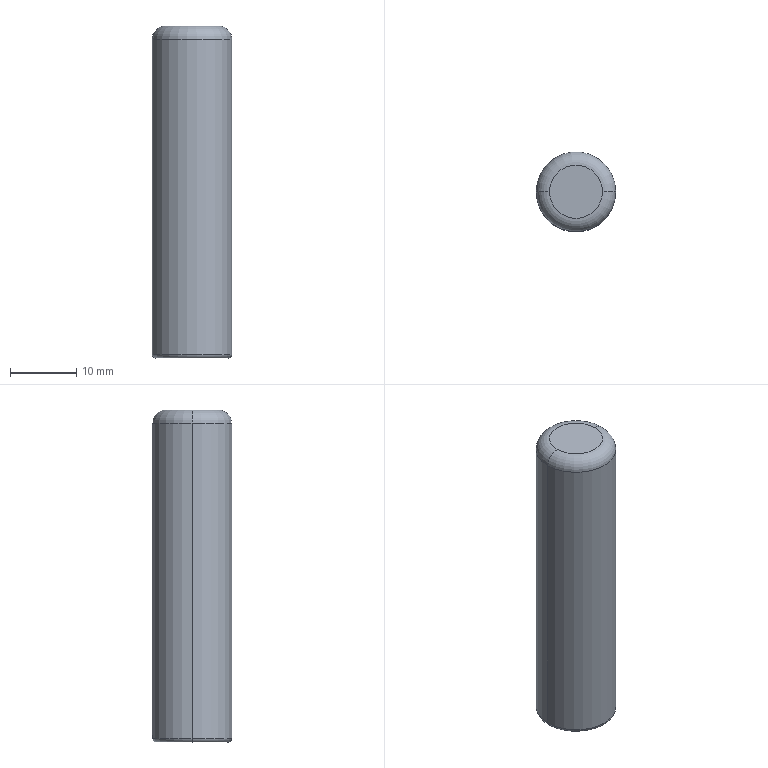Part | SolidWorks | features Fillet 2, Extrusion 1, ICE 1 | 1 solid | 10 faces | box 12 x 12 x 50 mm | volume 4836 mm3 | torus 4 | cylinder 4 | plane 2 | commonest cylinder face diameters 10 x2 12 x2
STEP:
#1=CARTESIAN_POINT('',(-6.,0.,48.));
#2=VERTEX_POINT('',#1);
#3=CARTESIAN_POINT('',(6.,0.,48.));
#4=VERTEX_POINT('',#3);
#5=CARTESIAN_POINT('',(0.,0.,48.));
#6=DIRECTION('',(0.,0.,-1.));
#7=DIRECTION('',(1.,0.,0.));
#8=AXIS2_PLACEMENT_3D('',#5,#6,#7);
#9=CIRCLE('',#8,6.);
#10=EDGE_CURVE('',#2,#4,#9,.T.);
#11=ORIENTED_EDGE('',*,*,#10,.F.);
#12=CARTESIAN_POINT('',(-4.,0.,50.));
#13=VERTEX_POINT('',#12);
#14=CARTESIAN_POINT('',(-4.,0.,48.));
#15=DIRECTION('',(0.,1.,0.));
#16=DIRECTION('',(-1.,0.,0.));
#17=AXIS2_PLACEMENT_3D('',#14,#15,#16);
#18=CIRCLE('',#17,2.);
#19=EDGE_CURVE('',#2,#13,#18,.T.);
#20=ORIENTED_EDGE('',*,*,#19,.T.);
#21=CARTESIAN_POINT('',(4.,0.,50.));
#22=VERTEX_POINT('',#21);
#23=CARTESIAN_POINT('',(0.,0.,50.));
#24=DIRECTION('',(0.,0.,1.));
#25=DIRECTION('',(1.,0.,0.));
#26=AXIS2_PLACEMENT_3D('',#23,#24,#25);
#27=CIRCLE('',#26,4.);
#28=EDGE_CURVE('',#22,#13,#27,.T.);
#29=ORIENTED_EDGE('',*,*,#28,.F.);
#30=CARTESIAN_POINT('',(4.,0.,48.));
#31=DIRECTION('',(0.,-1.,0.));
#32=DIRECTION('',(0.,0.,-1.));
#33=AXIS2_PLACEMENT_3D('',#30,#31,#32);
#34=CIRCLE('',#33,2.);
#35=EDGE_CURVE('',#4,#22,#34,.T.);
#36=ORIENTED_EDGE('',*,*,#35,.F.);
#37=EDGE_LOOP('',(#11,#20,#29,#36));
#38=FACE_OUTER_BOUND('',#37,.T.);
#39=CARTESIAN_POINT('',(0.,0.,48.));
#40=DIRECTION('',(0.,0.,1.));
#41=DIRECTION('',(1.,0.,0.));
#42=AXIS2_PLACEMENT_3D('',#39,#40,#41);
#43=TOROIDAL_SURFACE('',#42,4.,2.);
#44=ADVANCED_FACE('',(#38),#43,.T.);
#45=CARTESIAN_POINT('',(5.,0.,10.));
#46=VERTEX_POINT('',#45);
#47=CARTESIAN_POINT('',(-5.,0.,10.));
#48=VERTEX_POINT('',#47);
#49=CARTESIAN_POINT('',(0.,0.,10.));
#50=DIRECTION('',(0.,0.,-1.));
#51=DIRECTION('',(-1.,0.,0.));
#52=AXIS2_PLACEMENT_3D('',#49,#50,#51);
#53=CIRCLE('',#52,5.);
#54=EDGE_CURVE('',#46,#48,#53,.T.);
#55=ORIENTED_EDGE('',*,*,#54,.F.);
#56=CARTESIAN_POINT('',(5.,0.,0.5));
#57=VERTEX_POINT('',#56);
#58=CARTESIAN_POINT('',(5.,0.,10.));
#59=DIRECTION('',(0.,0.,-1.));
#60=VECTOR('',#59,1000.);
#61=LINE('',#58,#60);
#62=EDGE_CURVE('',#46,#57,#61,.T.);
#63=ORIENTED_EDGE('',*,*,#62,.T.);
#64=CARTESIAN_POINT('',(-5.,0.,0.5));
#65=VERTEX_POINT('',#64);
#66=CARTESIAN_POINT('',(0.,0.,0.5));
#67=DIRECTION('',(0.,0.,-1.));
#68=DIRECTION('',(-1.,0.,0.));
#69=AXIS2_PLACEMENT_3D('',#66,#67,#68);
#70=CIRCLE('',#69,5.);
#71=EDGE_CURVE('',#57,#65,#70,.T.);
#72=ORIENTED_EDGE('',*,*,#71,.T.);
#73=CARTESIAN_POINT('',(-5.,0.,10.));
#74=DIRECTION('',(0.,0.,-1.));
#75=VECTOR('',#74,1000.);
#76=LINE('',#73,#75);
#77=EDGE_CURVE('',#48,#65,#76,.T.);
#78=ORIENTED_EDGE('',*,*,#77,.F.);
#79=EDGE_LOOP('',(#55,#63,#72,#78));
#80=FACE_OUTER_BOUND('',#79,.T.);
#81=CARTESIAN_POINT('',(0.,0.,10.));
#82=DIRECTION('',(0.,0.,-1.));
#83=DIRECTION('',(-1.,0.,0.));
#84=AXIS2_PLACEMENT_3D('',#81,#82,#83);
#85=CYLINDRICAL_SURFACE('',#84,5.);
#86=ADVANCED_FACE('',(#80),#85,.F.);
#87=ORIENTED_EDGE('',*,*,#10,.T.);
#88=CARTESIAN_POINT('',(6.,0.,0.5));
#89=VERTEX_POINT('',#88);
#90=CARTESIAN_POINT('',(6.,0.,50.));
#91=DIRECTION('',(0.,0.,-1.));
#92=VECTOR('',#91,1000.);
#93=LINE('',#90,#92);
#94=EDGE_CURVE('',#4,#89,#93,.T.);
#95=ORIENTED_EDGE('',*,*,#94,.T.);
#96=CARTESIAN_POINT('',(-6.,0.,0.5));
#97=VERTEX_POINT('',#96);
#98=CARTESIAN_POINT('',(0.,0.,0.5));
#99=DIRECTION('',(0.,0.,1.));
#100=DIRECTION('',(-1.,0.,0.));
#101=AXIS2_PLACEMENT_3D('',#98,#99,#100);
#102=CIRCLE('',#101,6.);
#103=EDGE_CURVE('',#89,#97,#102,.T.);
#104=ORIENTED_EDGE('',*,*,#103,.T.);
#105=CARTESIAN_POINT('',(-6.,0.,50.));
#106=DIRECTION('',(0.,0.,-1.));
#107=VECTOR('',#106,1000.);
#108=LINE('',#105,#107);
#109=EDGE_CURVE('',#2,#97,#108,.T.);
#110=ORIENTED_EDGE('',*,*,#109,.F.);
#111=EDGE_LOOP('',(#87,#95,#104,#110));
#112=FACE_OUTER_BOUND('',#111,.T.);
#113=CARTESIAN_POINT('',(0.,0.,50.));
#114=DIRECTION('',(0.,0.,-1.));
#115=DIRECTION('',(-1.,0.,0.));
#116=AXIS2_PLACEMENT_3D('',#113,#114,#115);
#117=CYLINDRICAL_SURFACE('',#116,6.);
#118=ADVANCED_FACE('',(#112),#117,.T.);
#119=ORIENTED_EDGE('',*,*,#103,.F.);
#120=CARTESIAN_POINT('',(5.5,0.,0.5));
#121=DIRECTION('',(0.,1.,0.));
#122=DIRECTION('',(-1.,0.,0.));
#123=AXIS2_PLACEMENT_3D('',#120,#121,#122);
#124=CIRCLE('',#123,0.5);
#125=EDGE_CURVE('',#89,#57,#124,.T.);
#126=ORIENTED_EDGE('',*,*,#125,.T.);
#127=CARTESIAN_POINT('',(0.,0.,0.5));
#128=DIRECTION('',(0.,0.,-1.));
#129=DIRECTION('',(-1.,0.,0.));
#130=AXIS2_PLACEMENT_3D('',#127,#128,#129);
#131=CIRCLE('',#130,5.);
#132=EDGE_CURVE('',#65,#57,#131,.T.);
#133=ORIENTED_EDGE('',*,*,#132,.F.);
#134=CARTESIAN_POINT('',(-5.5,0.,0.5));
#135=DIRECTION('',(0.,-1.,0.));
#136=DIRECTION('',(0.,0.,-1.));
#137=AXIS2_PLACEMENT_3D('',#134,#135,#136);
#138=CIRCLE('',#137,0.5);
#139=EDGE_CURVE('',#97,#65,#138,.T.);
#140=ORIENTED_EDGE('',*,*,#139,.F.);
#141=EDGE_LOOP('',(#119,#126,#133,#140));
#142=FACE_OUTER_BOUND('',#141,.T.);
#143=CARTESIAN_POINT('',(0.,0.,0.5));
#144=DIRECTION('',(0.,0.,-1.));
#145=DIRECTION('',(-1.,0.,0.));
#146=AXIS2_PLACEMENT_3D('',#143,#144,#145);
#147=TOROIDAL_SURFACE('',#146,5.5,0.5);
#148=ADVANCED_FACE('',(#142),#147,.T.);
#149=ORIENTED_EDGE('',*,*,#125,.F.);
#150=CARTESIAN_POINT('',(0.,0.,0.5));
#151=DIRECTION('',(0.,0.,1.));
#152=DIRECTION('',(-1.,0.,0.));
#153=AXIS2_PLACEMENT_3D('',#150,#151,#152);
#154=CIRCLE('',#153,6.);
#155=EDGE_CURVE('',#97,#89,#154,.T.);
#156=ORIENTED_EDGE('',*,*,#155,.F.);
#157=ORIENTED_EDGE('',*,*,#139,.T.);
#158=ORIENTED_EDGE('',*,*,#71,.F.);
#159=EDGE_LOOP('',(#149,#156,#157,#158));
#160=FACE_OUTER_BOUND('',#159,.T.);
#161=CARTESIAN_POINT('',(0.,0.,0.5));
#162=DIRECTION('',(0.,0.,-1.));
#163=DIRECTION('',(-1.,0.,0.));
#164=AXIS2_PLACEMENT_3D('',#161,#162,#163);
#165=TOROIDAL_SURFACE('',#164,5.5,0.5);
#166=ADVANCED_FACE('',(#160),#165,.T.);
#167=ORIENTED_EDGE('',*,*,#94,.F.);
#168=CARTESIAN_POINT('',(0.,0.,48.));
#169=DIRECTION('',(0.,0.,-1.));
#170=DIRECTION('',(1.,0.,0.));
#171=AXIS2_PLACEMENT_3D('',#168,#169,#170);
#172=CIRCLE('',#171,6.);
#173=EDGE_CURVE('',#4,#2,#172,.T.);
#174=ORIENTED_EDGE('',*,*,#173,.T.);
#175=ORIENTED_EDGE('',*,*,#109,.T.);
#176=ORIENTED_EDGE('',*,*,#155,.T.);
#177=EDGE_LOOP('',(#167,#174,#175,#176));
#178=FACE_OUTER_BOUND('',#177,.T.);
#179=CARTESIAN_POINT('',(0.,0.,50.));
#180=DIRECTION('',(0.,0.,-1.));
#181=DIRECTION('',(-1.,0.,0.));
#182=AXIS2_PLACEMENT_3D('',#179,#180,#181);
#183=CYLINDRICAL_SURFACE('',#182,6.);
#184=ADVANCED_FACE('',(#178),#183,.T.);
#185=ORIENTED_EDGE('',*,*,#28,.T.);
#186=CARTESIAN_POINT('',(0.,0.,50.));
#187=DIRECTION('',(0.,0.,1.));
#188=DIRECTION('',(1.,0.,0.));
#189=AXIS2_PLACEMENT_3D('',#186,#187,#188);
#190=CIRCLE('',#189,4.);
#191=EDGE_CURVE('',#13,#22,#190,.T.);
#192=ORIENTED_EDGE('',*,*,#191,.T.);
#193=EDGE_LOOP('',(#185,#192));
#194=FACE_OUTER_BOUND('',#193,.T.);
#195=CARTESIAN_POINT('',(0.,0.,50.));
#196=DIRECTION('',(0.,0.,1.));
#197=DIRECTION('',(1.,0.,0.));
#198=AXIS2_PLACEMENT_3D('',#195,#196,#197);
#199=PLANE('',#198);
#200=ADVANCED_FACE('',(#194),#199,.T.);
#201=ORIENTED_EDGE('',*,*,#62,.F.);
#202=CARTESIAN_POINT('',(0.,0.,10.));
#203=DIRECTION('',(0.,0.,-1.));
#204=DIRECTION('',(-1.,0.,0.));
#205=AXIS2_PLACEMENT_3D('',#202,#203,#204);
#206=CIRCLE('',#205,5.);
#207=EDGE_CURVE('',#48,#46,#206,.T.);
#208=ORIENTED_EDGE('',*,*,#207,.F.);
#209=ORIENTED_EDGE('',*,*,#77,.T.);
#210=ORIENTED_EDGE('',*,*,#132,.T.);
#211=EDGE_LOOP('',(#201,#208,#209,#210));
#212=FACE_OUTER_BOUND('',#211,.T.);
#213=CARTESIAN_POINT('',(0.,0.,10.));
#214=DIRECTION('',(0.,0.,-1.));
#215=DIRECTION('',(-1.,0.,0.));
#216=AXIS2_PLACEMENT_3D('',#213,#214,#215);
#217=CYLINDRICAL_SURFACE('',#216,5.);
#218=ADVANCED_FACE('',(#212),#217,.F.);
#219=ORIENTED_EDGE('',*,*,#207,.T.);
#220=ORIENTED_EDGE('',*,*,#54,.T.);
#221=EDGE_LOOP('',(#219,#220));
#222=FACE_OUTER_BOUND('',#221,.T.);
#223=CARTESIAN_POINT('',(0.,0.,10.));
#224=DIRECTION('',(0.,0.,-1.));
#225=DIRECTION('',(-1.,0.,0.));
#226=AXIS2_PLACEMENT_3D('',#223,#224,#225);
#227=PLANE('',#226);
#228=ADVANCED_FACE('',(#222),#227,.T.);
#229=ORIENTED_EDGE('',*,*,#19,.F.);
#230=ORIENTED_EDGE('',*,*,#173,.F.);
#231=ORIENTED_EDGE('',*,*,#35,.T.);
#232=ORIENTED_EDGE('',*,*,#191,.F.);
#233=EDGE_LOOP('',(#229,#230,#231,#232));
#234=FACE_OUTER_BOUND('',#233,.T.);
#235=CARTESIAN_POINT('',(0.,0.,48.));
#236=DIRECTION('',(0.,0.,1.));
#237=DIRECTION('',(1.,0.,0.));
#238=AXIS2_PLACEMENT_3D('',#235,#236,#237);
#239=TOROIDAL_SURFACE('',#238,4.,2.);
#240=ADVANCED_FACE('',(#234),#239,.T.);
#241=CLOSED_SHELL('',(#44,#86,#118,#148,#166,#184,#200,#218,#228,#240));
#242=MANIFOLD_SOLID_BREP('',#241);
#243=CARTESIAN_POINT('',(0.,0.,0.));
#244=DIRECTION('',(0.,0.,1.));
#245=DIRECTION('',(1.,0.,0.));
#246=AXIS2_PLACEMENT_3D('',#243,#244,#245);
#247=(LENGTH_UNIT()NAMED_UNIT(*)SI_UNIT(.MILLI.,.METRE.));
#248=UNCERTAINTY_MEASURE_WITH_UNIT(LENGTH_MEASURE(0.00001),#247,'','');
#249=(NAMED_UNIT(*)PLANE_ANGLE_UNIT()SI_UNIT($,.RADIAN.));
#250=(NAMED_UNIT(*)SI_UNIT($,.STERADIAN.)SOLID_ANGLE_UNIT());
#251=(GEOMETRIC_REPRESENTATION_CONTEXT(3)GLOBAL_UNCERTAINTY_ASSIGNED_CONTEXT((#248))GLOBAL_UNIT_ASSIGNED_CONTEXT((#247,#249,#250))REPRESENTATION_CONTEXT('',''));
#252=ADVANCED_BREP_SHAPE_REPRESENTATION('',(#242,#246),#251);